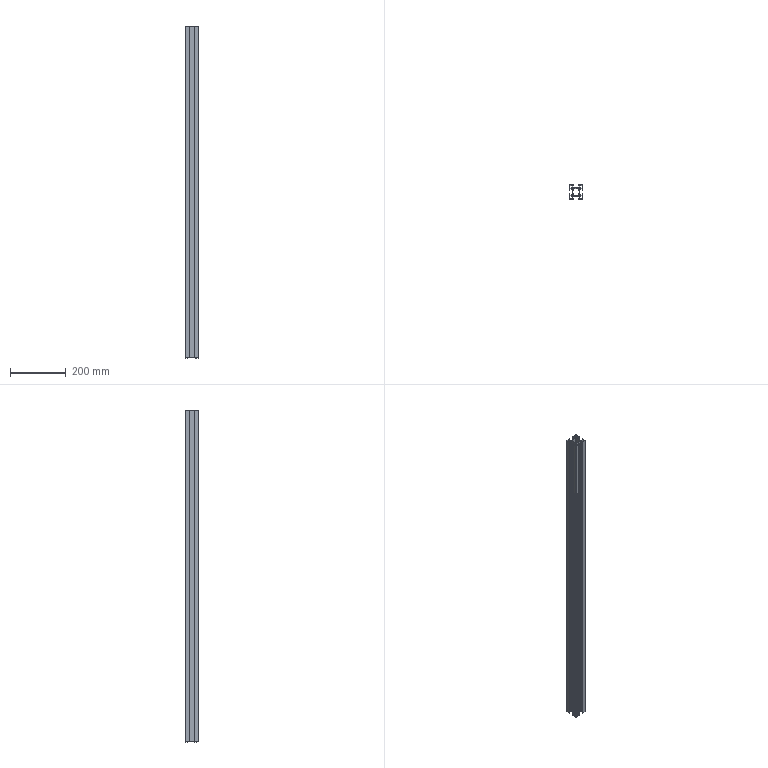Part | STEP file | 46A-00006CC11-1195mm | 1 solid | 142 faces | box 50 x 50 x 1195 mm | volume 702053 mm3 | cylinder 84 | plane 58 | commonest cylinder face diameters 1 x24 4 x24 1.5 x16 3.7 x8 6.7 x8 2 x4